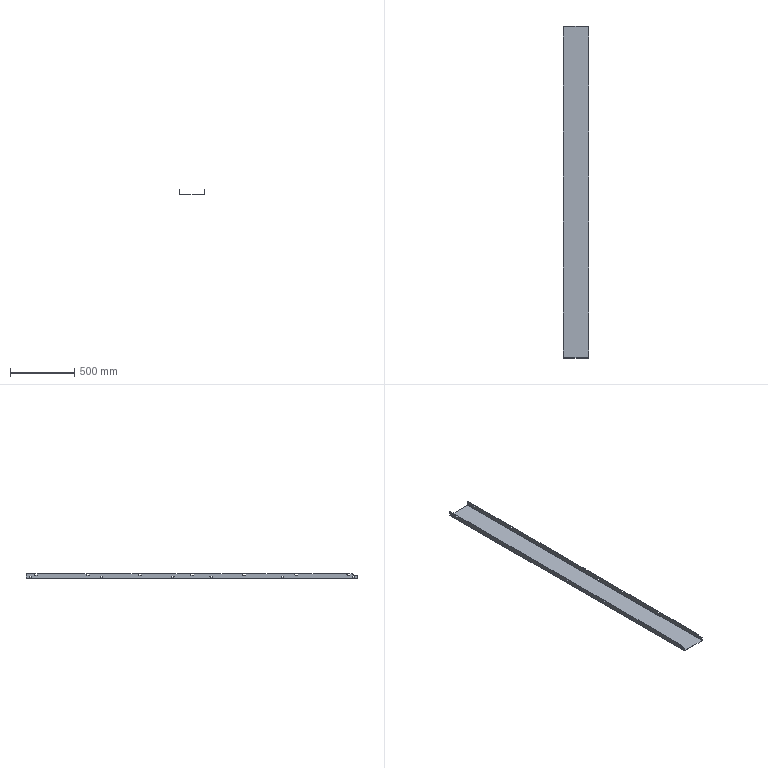Part | 1 solid | 162 faces | box 195 x 2576 x 38.5 mm | volume 824417 mm3 | plane 116 | cylinder 46 | commonest cylinder face diameters 6.4 x24 8.5 x14 10 x4 0.4 x2 2.8 x2